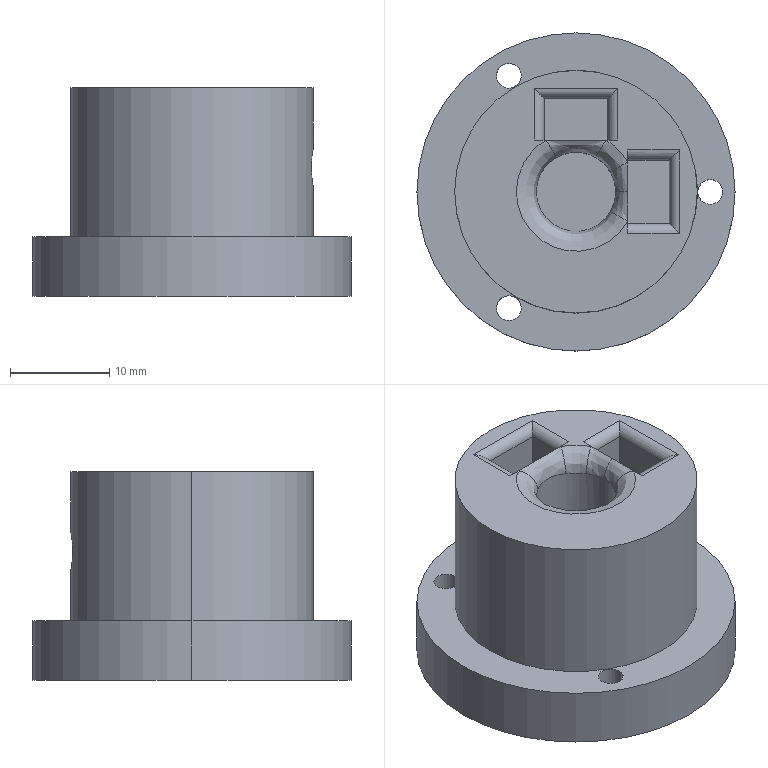Part | SolidWorks | 2 solids | 53 faces | box 32 x 32 x 21 mm | volume 10117 mm3 | cylinder 26 | spline 15 | plane 12 | commonest cylinder face diameters 2.4 x8 2 x6 2.5 x6 8 x2 24.4 x2 32 x2